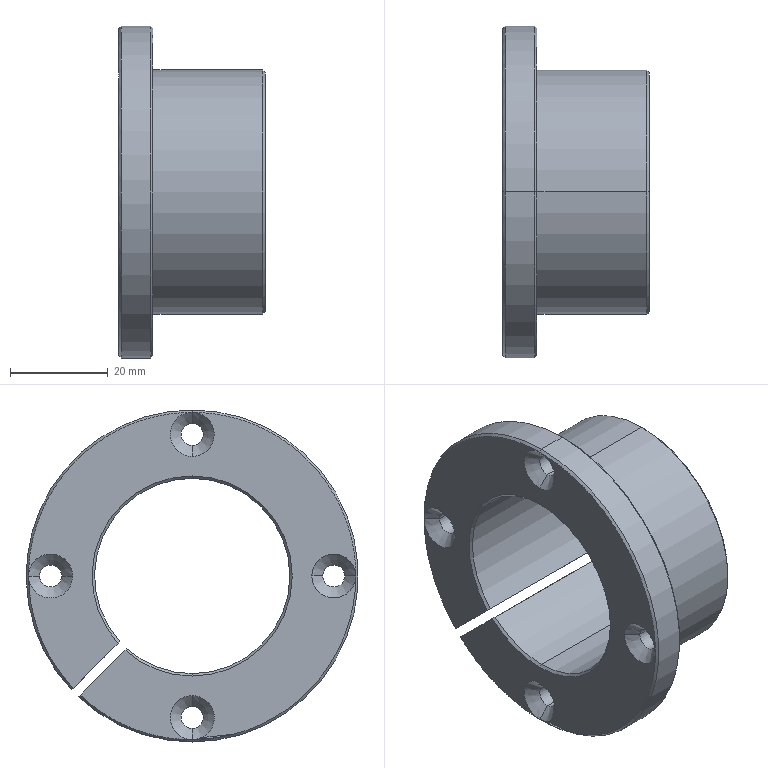Part | SolidWorks | features ICE 2, MoveFace 2, Chamfer 1, CirPattern 1, DelFace 1, RevCut 1, Revolution 1 | 1 solid | 45 faces | box 30 x 68 x 68 mm | volume 31718 mm3 | cone 23 | cylinder 17 | plane 5 | commonest cylinder face diameters 4.5 x8 40 x3 50 x3 68 x3
STEP:
#1=CARTESIAN_POINT('',(25.,0.,-24.5));
#2=VERTEX_POINT('',#1);
#3=CARTESIAN_POINT('',(25.,16.603,-18.017));
#4=VERTEX_POINT('',#3);
#5=CARTESIAN_POINT('',(25.,0.,0.));
#6=DIRECTION('',(1.,0.,0.));
#7=DIRECTION('',(0.,0.,-1.));
#8=AXIS2_PLACEMENT_3D('',#5,#6,#7);
#9=CIRCLE('',#8,24.5);
#10=EDGE_CURVE('',#2,#4,#9,.T.);
#11=ORIENTED_EDGE('',*,*,#10,.F.);
#12=CARTESIAN_POINT('',(24.5,0.,-25.));
#13=VERTEX_POINT('',#12);
#14=CARTESIAN_POINT('',(24.5,0.,-25.));
#15=DIRECTION('',(-0.7071,0.,-0.7071));
#16=VECTOR('',#15,1000.);
#17=LINE('',#14,#16);
#18=EDGE_CURVE('',#2,#13,#17,.T.);
#19=ORIENTED_EDGE('',*,*,#18,.T.);
#20=CARTESIAN_POINT('',(24.5,16.956,-18.371));
#21=VERTEX_POINT('',#20);
#22=CARTESIAN_POINT('',(24.5,0.,0.));
#23=DIRECTION('',(-1.,0.,0.));
#24=DIRECTION('',(0.,0.,-1.));
#25=AXIS2_PLACEMENT_3D('',#22,#23,#24);
#26=CIRCLE('',#25,25.);
#27=EDGE_CURVE('',#21,#13,#26,.T.);
#28=ORIENTED_EDGE('',*,*,#27,.F.);
#29=CARTESIAN_POINT('',(25.,16.603,-18.017));
#30=CARTESIAN_POINT('',(24.833,16.721,-18.135));
#31=CARTESIAN_POINT('',(24.667,16.838,-18.253));
#32=CARTESIAN_POINT('',(24.5,16.956,-18.371));
#33=B_SPLINE_CURVE_WITH_KNOTS('',3,(#29,#30,#31,#32),.UNSPECIFIED.,.F.,.F.,(4,4),(0.,0.0007074),.UNSPECIFIED.);
#34=EDGE_CURVE('',#4,#21,#33,.T.);
#35=ORIENTED_EDGE('',*,*,#34,.F.);
#36=EDGE_LOOP('',(#11,#19,#28,#35));
#37=FACE_OUTER_BOUND('',#36,.T.);
#38=CARTESIAN_POINT('',(24.5,0.,0.));
#39=DIRECTION('',(-1.,0.,0.));
#40=DIRECTION('',(0.,0.,1.));
#41=AXIS2_PLACEMENT_3D('',#38,#39,#40);
#42=CONICAL_SURFACE('',#41,25.,0.7854);
#43=ADVANCED_FACE('',(#37),#42,.T.);
#44=ORIENTED_EDGE('',*,*,#18,.F.);
#45=CARTESIAN_POINT('',(25.,0.,24.5));
#46=VERTEX_POINT('',#45);
#47=CARTESIAN_POINT('',(25.,0.,0.));
#48=DIRECTION('',(1.,0.,0.));
#49=DIRECTION('',(0.,0.,-1.));
#50=AXIS2_PLACEMENT_3D('',#47,#48,#49);
#51=CIRCLE('',#50,24.5);
#52=EDGE_CURVE('',#46,#2,#51,.T.);
#53=ORIENTED_EDGE('',*,*,#52,.F.);
#54=CARTESIAN_POINT('',(24.5,0.,25.));
#55=VERTEX_POINT('',#54);
#56=CARTESIAN_POINT('',(24.5,0.,25.));
#57=DIRECTION('',(-0.7071,0.,0.7071));
#58=VECTOR('',#57,1000.);
#59=LINE('',#56,#58);
#60=EDGE_CURVE('',#46,#55,#59,.T.);
#61=ORIENTED_EDGE('',*,*,#60,.T.);
#62=CARTESIAN_POINT('',(24.5,0.,0.));
#63=DIRECTION('',(-1.,0.,0.));
#64=DIRECTION('',(0.,0.,-1.));
#65=AXIS2_PLACEMENT_3D('',#62,#63,#64);
#66=CIRCLE('',#65,25.);
#67=EDGE_CURVE('',#13,#55,#66,.T.);
#68=ORIENTED_EDGE('',*,*,#67,.F.);
#69=EDGE_LOOP('',(#44,#53,#61,#68));
#70=FACE_OUTER_BOUND('',#69,.T.);
#71=CARTESIAN_POINT('',(24.5,0.,0.));
#72=DIRECTION('',(-1.,0.,0.));
#73=DIRECTION('',(0.,0.,1.));
#74=AXIS2_PLACEMENT_3D('',#71,#72,#73);
#75=CONICAL_SURFACE('',#74,25.,0.7854);
#76=ADVANCED_FACE('',(#70),#75,.T.);
#77=CARTESIAN_POINT('',(24.5,0.,20.));
#78=VERTEX_POINT('',#77);
#79=CARTESIAN_POINT('',(24.5,0.,-20.));
#80=VERTEX_POINT('',#79);
#81=CARTESIAN_POINT('',(24.5,0.,0.));
#82=DIRECTION('',(1.,0.,0.));
#83=DIRECTION('',(0.,0.,-1.));
#84=AXIS2_PLACEMENT_3D('',#81,#82,#83);
#85=CIRCLE('',#84,20.);
#86=EDGE_CURVE('',#78,#80,#85,.T.);
#87=ORIENTED_EDGE('',*,*,#86,.F.);
#88=CARTESIAN_POINT('',(25.,0.,20.5));
#89=VERTEX_POINT('',#88);
#90=CARTESIAN_POINT('',(24.5,0.,20.));
#91=DIRECTION('',(0.7071,0.,0.7071));
#92=VECTOR('',#91,1000.);
#93=LINE('',#90,#92);
#94=EDGE_CURVE('',#78,#89,#93,.T.);
#95=ORIENTED_EDGE('',*,*,#94,.T.);
#96=CARTESIAN_POINT('',(25.,0.,-20.5));
#97=VERTEX_POINT('',#96);
#98=CARTESIAN_POINT('',(25.,0.,0.));
#99=DIRECTION('',(-1.,0.,0.));
#100=DIRECTION('',(0.,0.,-1.));
#101=AXIS2_PLACEMENT_3D('',#98,#99,#100);
#102=CIRCLE('',#101,20.5);
#103=EDGE_CURVE('',#97,#89,#102,.T.);
#104=ORIENTED_EDGE('',*,*,#103,.F.);
#105=CARTESIAN_POINT('',(24.5,0.,-20.));
#106=DIRECTION('',(0.7071,0.,-0.7071));
#107=VECTOR('',#106,1000.);
#108=LINE('',#105,#107);
#109=EDGE_CURVE('',#80,#97,#108,.T.);
#110=ORIENTED_EDGE('',*,*,#109,.F.);
#111=EDGE_LOOP('',(#87,#95,#104,#110));
#112=FACE_OUTER_BOUND('',#111,.T.);
#113=CARTESIAN_POINT('',(24.5,0.,0.));
#114=DIRECTION('',(1.,0.,0.));
#115=DIRECTION('',(0.,0.,-1.));
#116=AXIS2_PLACEMENT_3D('',#113,#114,#115);
#117=CONICAL_SURFACE('',#116,20.,0.7854);
#118=ADVANCED_FACE('',(#112),#117,.F.);
#119=CARTESIAN_POINT('',(24.5,13.417,-14.832));
#120=VERTEX_POINT('',#119);
#121=CARTESIAN_POINT('',(24.5,0.,0.));
#122=DIRECTION('',(1.,0.,0.));
#123=DIRECTION('',(0.,0.,-1.));
#124=AXIS2_PLACEMENT_3D('',#121,#122,#123);
#125=CIRCLE('',#124,20.);
#126=EDGE_CURVE('',#80,#120,#125,.T.);
#127=ORIENTED_EDGE('',*,*,#126,.F.);
#128=ORIENTED_EDGE('',*,*,#109,.T.);
#129=CARTESIAN_POINT('',(25.,13.771,-15.186));
#130=VERTEX_POINT('',#129);
#131=CARTESIAN_POINT('',(25.,0.,0.));
#132=DIRECTION('',(-1.,0.,0.));
#133=DIRECTION('',(0.,0.,-1.));
#134=AXIS2_PLACEMENT_3D('',#131,#132,#133);
#135=CIRCLE('',#134,20.5);
#136=EDGE_CURVE('',#130,#97,#135,.T.);
#137=ORIENTED_EDGE('',*,*,#136,.F.);
#138=CARTESIAN_POINT('',(24.5,13.417,-14.832));
#139=CARTESIAN_POINT('',(24.667,13.535,-14.95));
#140=CARTESIAN_POINT('',(24.833,13.653,-15.068));
#141=CARTESIAN_POINT('',(25.,13.771,-15.186));
#142=B_SPLINE_CURVE_WITH_KNOTS('',3,(#138,#139,#140,#141),.UNSPECIFIED.,.F.,.F.,(4,4),(0.,0.0007075),.UNSPECIFIED.);
#143=EDGE_CURVE('',#120,#130,#142,.T.);
#144=ORIENTED_EDGE('',*,*,#143,.F.);
#145=EDGE_LOOP('',(#127,#128,#137,#144));
#146=FACE_OUTER_BOUND('',#145,.T.);
#147=CARTESIAN_POINT('',(24.5,0.,0.));
#148=DIRECTION('',(1.,0.,0.));
#149=DIRECTION('',(0.,0.,-1.));
#150=AXIS2_PLACEMENT_3D('',#147,#148,#149);
#151=CONICAL_SURFACE('',#150,20.,0.7854);
#152=ADVANCED_FACE('',(#146),#151,.F.);
#153=CARTESIAN_POINT('',(2.,0.,-33.5));
#154=VERTEX_POINT('',#153);
#155=CARTESIAN_POINT('',(2.,22.97,-24.385));
#156=VERTEX_POINT('',#155);
#157=CARTESIAN_POINT('',(2.,0.,0.));
#158=DIRECTION('',(1.,0.,0.));
#159=DIRECTION('',(0.,0.,-1.));
#160=AXIS2_PLACEMENT_3D('',#157,#158,#159);
#161=CIRCLE('',#160,33.5);
#162=EDGE_CURVE('',#154,#156,#161,.T.);
#163=ORIENTED_EDGE('',*,*,#162,.F.);
#164=CARTESIAN_POINT('',(1.5,0.,-34.));
#165=VERTEX_POINT('',#164);
#166=CARTESIAN_POINT('',(2.,0.,-33.5));
#167=DIRECTION('',(-0.7071,0.,-0.7071));
#168=VECTOR('',#167,1000.);
#169=LINE('',#166,#168);
#170=EDGE_CURVE('',#154,#165,#169,.T.);
#171=ORIENTED_EDGE('',*,*,#170,.T.);
#172=CARTESIAN_POINT('',(1.5,23.324,-24.738));
#173=VERTEX_POINT('',#172);
#174=CARTESIAN_POINT('',(1.5,0.,0.));
#175=DIRECTION('',(-1.,0.,0.));
#176=DIRECTION('',(0.,0.,-1.));
#177=AXIS2_PLACEMENT_3D('',#174,#175,#176);
#178=CIRCLE('',#177,34.);
#179=EDGE_CURVE('',#173,#165,#178,.T.);
#180=ORIENTED_EDGE('',*,*,#179,.F.);
#181=CARTESIAN_POINT('',(2.,22.97,-24.385));
#182=CARTESIAN_POINT('',(1.833,23.088,-24.503));
#183=CARTESIAN_POINT('',(1.667,23.206,-24.62));
#184=CARTESIAN_POINT('',(1.5,23.324,-24.738));
#185=B_SPLINE_CURVE_WITH_KNOTS('',3,(#181,#182,#183,#184),.UNSPECIFIED.,.F.,.F.,(4,4),(0.,0.0007073),.UNSPECIFIED.);
#186=EDGE_CURVE('',#156,#173,#185,.T.);
#187=ORIENTED_EDGE('',*,*,#186,.F.);
#188=EDGE_LOOP('',(#163,#171,#180,#187));
#189=FACE_OUTER_BOUND('',#188,.T.);
#190=CARTESIAN_POINT('',(2.,0.,0.));
#191=DIRECTION('',(-1.,0.,0.));
#192=DIRECTION('',(0.,0.,1.));
#193=AXIS2_PLACEMENT_3D('',#190,#191,#192);
#194=CONICAL_SURFACE('',#193,33.5,0.7854);
#195=ADVANCED_FACE('',(#189),#194,.T.);
#196=ORIENTED_EDGE('',*,*,#170,.F.);
#197=CARTESIAN_POINT('',(2.,0.,33.5));
#198=VERTEX_POINT('',#197);
#199=CARTESIAN_POINT('',(2.,0.,0.));
#200=DIRECTION('',(1.,0.,0.));
#201=DIRECTION('',(0.,0.,-1.));
#202=AXIS2_PLACEMENT_3D('',#199,#200,#201);
#203=CIRCLE('',#202,33.5);
#204=EDGE_CURVE('',#198,#154,#203,.T.);
#205=ORIENTED_EDGE('',*,*,#204,.F.);
#206=CARTESIAN_POINT('',(1.5,0.,34.));
#207=VERTEX_POINT('',#206);
#208=CARTESIAN_POINT('',(2.,0.,33.5));
#209=DIRECTION('',(-0.7071,0.,0.7071));
#210=VECTOR('',#209,1000.);
#211=LINE('',#208,#210);
#212=EDGE_CURVE('',#198,#207,#211,.T.);
#213=ORIENTED_EDGE('',*,*,#212,.T.);
#214=CARTESIAN_POINT('',(1.5,0.,0.));
#215=DIRECTION('',(-1.,0.,0.));
#216=DIRECTION('',(0.,0.,-1.));
#217=AXIS2_PLACEMENT_3D('',#214,#215,#216);
#218=CIRCLE('',#217,34.);
#219=EDGE_CURVE('',#165,#207,#218,.T.);
#220=ORIENTED_EDGE('',*,*,#219,.F.);
#221=EDGE_LOOP('',(#196,#205,#213,#220));
#222=FACE_OUTER_BOUND('',#221,.T.);
#223=CARTESIAN_POINT('',(2.,0.,0.));
#224=DIRECTION('',(-1.,0.,0.));
#225=DIRECTION('',(0.,0.,1.));
#226=AXIS2_PLACEMENT_3D('',#223,#224,#225);
#227=CONICAL_SURFACE('',#226,33.5,0.7854);
#228=ADVANCED_FACE('',(#222),#227,.T.);
#229=CARTESIAN_POINT('',(-5.,0.,33.5));
#230=VERTEX_POINT('',#229);
#231=CARTESIAN_POINT('',(-5.,33.5,0.));
#232=VERTEX_POINT('',#231);
#233=CARTESIAN_POINT('',(-5.,0.,0.));
#234=DIRECTION('',(-1.,0.,0.));
#235=DIRECTION('',(0.,0.,1.));
#236=AXIS2_PLACEMENT_3D('',#233,#234,#235);
#237=CIRCLE('',#236,33.5);
#238=EDGE_CURVE('',#230,#232,#237,.T.);
#239=ORIENTED_EDGE('',*,*,#238,.F.);
#240=CARTESIAN_POINT('',(-4.5,0.,34.));
#241=VERTEX_POINT('',#240);
#242=CARTESIAN_POINT('',(-5.,0.,33.5));
#243=DIRECTION('',(0.7071,0.,0.7071));
#244=VECTOR('',#243,1000.);
#245=LINE('',#242,#244);
#246=EDGE_CURVE('',#230,#241,#245,.T.);
#247=ORIENTED_EDGE('',*,*,#246,.T.);
#248=CARTESIAN_POINT('',(-4.5,24.738,-23.324));
#249=VERTEX_POINT('',#248);
#250=CARTESIAN_POINT('',(-4.5,0.,0.));
#251=DIRECTION('',(1.,0.,0.));
#252=DIRECTION('',(0.,0.,1.));
#253=AXIS2_PLACEMENT_3D('',#250,#251,#252);
#254=CIRCLE('',#253,34.);
#255=EDGE_CURVE('',#249,#241,#254,.T.);
#256=ORIENTED_EDGE('',*,*,#255,.F.);
#257=CARTESIAN_POINT('',(-5.,24.385,-22.97));
#258=VERTEX_POINT('',#257);
#259=CARTESIAN_POINT('',(-5.,24.385,-22.97));
#260=CARTESIAN_POINT('',(-4.833,24.503,-23.088));
#261=CARTESIAN_POINT('',(-4.667,24.62,-23.206));
#262=CARTESIAN_POINT('',(-4.5,24.738,-23.324));
#263=B_SPLINE_CURVE_WITH_KNOTS('',3,(#259,#260,#261,#262),.UNSPECIFIED.,.F.,.F.,(4,4),(0.,0.0007073),.UNSPECIFIED.);
#264=EDGE_CURVE('',#258,#249,#263,.T.);
#265=ORIENTED_EDGE('',*,*,#264,.F.);
#266=CARTESIAN_POINT('',(-5.,0.,0.));
#267=DIRECTION('',(-1.,0.,0.));
#268=DIRECTION('',(0.,0.,1.));
#269=AXIS2_PLACEMENT_3D('',#266,#267,#268);
#270=CIRCLE('',#269,33.5);
#271=EDGE_CURVE('',#232,#258,#270,.T.);
#272=ORIENTED_EDGE('',*,*,#271,.F.);
#273=EDGE_LOOP('',(#239,#247,#256,#265,#272));
#274=FACE_OUTER_BOUND('',#273,.T.);
#275=CARTESIAN_POINT('',(-5.,0.,0.));
#276=DIRECTION('',(1.,0.,0.));
#277=DIRECTION('',(0.,0.,-1.));
#278=AXIS2_PLACEMENT_3D('',#275,#276,#277);
#279=CONICAL_SURFACE('',#278,33.5,0.7854);
#280=ADVANCED_FACE('',(#274),#279,.T.);
#281=ORIENTED_EDGE('',*,*,#246,.F.);
#282=CARTESIAN_POINT('',(-5.,-33.5,0.));
#283=VERTEX_POINT('',#282);
#284=CARTESIAN_POINT('',(-5.,0.,0.));
#285=DIRECTION('',(-1.,0.,0.));
#286=DIRECTION('',(0.,0.,1.));
#287=AXIS2_PLACEMENT_3D('',#284,#285,#286);
#288=CIRCLE('',#287,33.5);
#289=EDGE_CURVE('',#283,#230,#288,.T.);
#290=ORIENTED_EDGE('',*,*,#289,.F.);
#291=CARTESIAN_POINT('',(-5.,0.,-33.5));
#292=VERTEX_POINT('',#291);
#293=CARTESIAN_POINT('',(-5.,0.,0.));
#294=DIRECTION('',(-1.,0.,0.));
#295=DIRECTION('',(0.,0.,1.));
#296=AXIS2_PLACEMENT_3D('',#293,#294,#295);
#297=CIRCLE('',#296,33.5);
#298=EDGE_CURVE('',#292,#283,#297,.T.);
#299=ORIENTED_EDGE('',*,*,#298,.F.);
#300=CARTESIAN_POINT('',(-4.5,0.,-34.));
#301=VERTEX_POINT('',#300);
#302=CARTESIAN_POINT('',(-5.,0.,-33.5));
#303=DIRECTION('',(0.7071,0.,-0.7071));
#304=VECTOR('',#303,1000.);
#305=LINE('',#302,#304);
#306=EDGE_CURVE('',#292,#301,#305,.T.);
#307=ORIENTED_EDGE('',*,*,#306,.T.);
#308=CARTESIAN_POINT('',(-4.5,0.,0.));
#309=DIRECTION('',(1.,0.,0.));
#310=DIRECTION('',(0.,0.,1.));
#311=AXIS2_PLACEMENT_3D('',#308,#309,#310);
#312=CIRCLE('',#311,34.);
#313=EDGE_CURVE('',#241,#301,#312,.T.);
#314=ORIENTED_EDGE('',*,*,#313,.F.);
#315=EDGE_LOOP('',(#281,#290,#299,#307,#314));
#316=FACE_OUTER_BOUND('',#315,.T.);
#317=CARTESIAN_POINT('',(-5.,0.,0.));
#318=DIRECTION('',(1.,0.,0.));
#319=DIRECTION('',(0.,0.,-1.));
#320=AXIS2_PLACEMENT_3D('',#317,#318,#319);
#321=CONICAL_SURFACE('',#320,33.5,0.7854);
#322=ADVANCED_FACE('',(#316),#321,.T.);
#323=CARTESIAN_POINT('',(-4.5,0.,-20.));
#324=VERTEX_POINT('',#323);
#325=CARTESIAN_POINT('',(-4.5,0.,20.));
#326=VERTEX_POINT('',#325);
#327=CARTESIAN_POINT('',(-4.5,0.,0.));
#328=DIRECTION('',(-1.,0.,0.));
#329=DIRECTION('',(0.,0.,1.));
#330=AXIS2_PLACEMENT_3D('',#327,#328,#329);
#331=CIRCLE('',#330,20.);
#332=EDGE_CURVE('',#324,#326,#331,.T.);
#333=ORIENTED_EDGE('',*,*,#332,.F.);
#334=CARTESIAN_POINT('',(-5.,0.,-20.5));
#335=VERTEX_POINT('',#334);
#336=CARTESIAN_POINT('',(-4.5,0.,-20.));
#337=DIRECTION('',(-0.7071,0.,-0.7071));
#338=VECTOR('',#337,1000.);
#339=LINE('',#336,#338);
#340=EDGE_CURVE('',#324,#335,#339,.T.);
#341=ORIENTED_EDGE('',*,*,#340,.T.);
#342=CARTESIAN_POINT('',(-5.,0.,20.5));
#343=VERTEX_POINT('',#342);
#344=CARTESIAN_POINT('',(-5.,0.,0.));
#345=DIRECTION('',(1.,0.,0.));
#346=DIRECTION('',(0.,0.,1.));
#347=AXIS2_PLACEMENT_3D('',#344,#345,#346);
#348=CIRCLE('',#347,20.5);
#349=EDGE_CURVE('',#343,#335,#348,.T.);
#350=ORIENTED_EDGE('',*,*,#349,.F.);
#351=CARTESIAN_POINT('',(-4.5,0.,20.));
#352=DIRECTION('',(-0.7071,0.,0.7071));
#353=VECTOR('',#352,1000.);
#354=LINE('',#351,#353);
#355=EDGE_CURVE('',#326,#343,#354,.T.);
#356=ORIENTED_EDGE('',*,*,#355,.F.);
#357=EDGE_LOOP('',(#333,#341,#350,#356));
#358=FACE_OUTER_BOUND('',#357,.T.);
#359=CARTESIAN_POINT('',(-4.5,0.,0.));
#360=DIRECTION('',(-1.,0.,0.));
#361=DIRECTION('',(0.,0.,1.));
#362=AXIS2_PLACEMENT_3D('',#359,#360,#361);
#363=CONICAL_SURFACE('',#362,20.,0.7854);
#364=ADVANCED_FACE('',(#358),#363,.F.);
#365=CARTESIAN_POINT('',(-4.5,14.832,-13.417));
#366=VERTEX_POINT('',#365);
#367=CARTESIAN_POINT('',(-4.5,0.,0.));
#368=DIRECTION('',(-1.,0.,0.));
#369=DIRECTION('',(0.,0.,1.));
#370=AXIS2_PLACEMENT_3D('',#367,#368,#369);
#371=CIRCLE('',#370,20.);
#372=EDGE_CURVE('',#326,#366,#371,.T.);
#373=ORIENTED_EDGE('',*,*,#372,.F.);
#374=ORIENTED_EDGE('',*,*,#355,.T.);
#375=CARTESIAN_POINT('',(-5.,15.186,-13.771));
#376=VERTEX_POINT('',#375);
#377=CARTESIAN_POINT('',(-5.,0.,0.));
#378=DIRECTION('',(1.,0.,0.));
#379=DIRECTION('',(0.,0.,1.));
#380=AXIS2_PLACEMENT_3D('',#377,#378,#379);
#381=CIRCLE('',#380,20.5);
#382=EDGE_CURVE('',#376,#343,#381,.T.);
#383=ORIENTED_EDGE('',*,*,#382,.F.);
#384=CARTESIAN_POINT('',(-4.5,14.832,-13.417));
#385=CARTESIAN_POINT('',(-4.667,14.95,-13.535));
#386=CARTESIAN_POINT('',(-4.833,15.068,-13.653));
#387=CARTESIAN_POINT('',(-5.,15.186,-13.771));
#388=B_SPLINE_CURVE_WITH_KNOTS('',3,(#384,#385,#386,#387),.UNSPECIFIED.,.F.,.F.,(4,4),(0.,0.0007075),.UNSPECIFIED.);
#389=EDGE_CURVE('',#366,#376,#388,.T.);
#390=ORIENTED_EDGE('',*,*,#389,.F.);
#391=EDGE_LOOP('',(#373,#374,#383,#390));
#392=FACE_OUTER_BOUND('',#391,.T.);
#393=CARTESIAN_POINT('',(-4.5,0.,0.));
#394=DIRECTION('',(-1.,0.,0.));
#395=DIRECTION('',(0.,0.,1.));
#396=AXIS2_PLACEMENT_3D('',#393,#394,#395);
#397=CONICAL_SURFACE('',#396,20.,0.7854);
#398=ADVANCED_FACE('',(#392),#397,.F.);
#399=ORIENTED_EDGE('',*,*,#179,.T.);
#400=CARTESIAN_POINT('',(5.,0.,-34.));
#401=DIRECTION('',(-1.,0.,0.));
#402=VECTOR('',#401,1000.);
#403=LINE('',#400,#402);
#404=EDGE_CURVE('',#165,#301,#403,.T.);
#405=ORIENTED_EDGE('',*,*,#404,.T.);
#406=CARTESIAN_POINT('',(-4.5,23.324,-24.738));
#407=VERTEX_POINT('',#406);
#408=CARTESIAN_POINT('',(-4.5,0.,0.));
#409=DIRECTION('',(1.,0.,0.));
#410=DIRECTION('',(0.,0.,1.));
#411=AXIS2_PLACEMENT_3D('',#408,#409,#410);
#412=CIRCLE('',#411,34.);
#413=EDGE_CURVE('',#301,#407,#412,.T.);
#414=ORIENTED_EDGE('',*,*,#413,.T.);
#415=CARTESIAN_POINT('',(5.,23.324,-24.738));
#416=DIRECTION('',(1.,0.,0.));
#417=VECTOR('',#416,1000.);
#418=LINE('',#415,#417);
#419=EDGE_CURVE('',#407,#173,#418,.T.);
#420=ORIENTED_EDGE('',*,*,#419,.T.);
#421=EDGE_LOOP('',(#399,#405,#414,#420));
#422=FACE_OUTER_BOUND('',#421,.T.);
#423=CARTESIAN_POINT('',(5.,0.,0.));
#424=DIRECTION('',(-1.,0.,0.));
#425=DIRECTION('',(0.,0.,1.));
#426=AXIS2_PLACEMENT_3D('',#423,#424,#425);
#427=CYLINDRICAL_SURFACE('',#426,34.);
#428=ADVANCED_FACE('',(#422),#427,.T.);
#429=ORIENTED_EDGE('',*,*,#404,.F.);
#430=ORIENTED_EDGE('',*,*,#219,.T.);
#431=CARTESIAN_POINT('',(5.,0.,34.));
#432=DIRECTION('',(-1.,0.,0.));
#433=VECTOR('',#432,1000.);
#434=LINE('',#431,#433);
#435=EDGE_CURVE('',#207,#241,#434,.T.);
#436=ORIENTED_EDGE('',*,*,#435,.T.);
#437=ORIENTED_EDGE('',*,*,#313,.T.);
#438=EDGE_LOOP('',(#429,#430,#436,#437));
#439=FACE_OUTER_BOUND('',#438,.T.);
#440=CARTESIAN_POINT('',(5.,0.,0.));
#441=DIRECTION('',(-1.,0.,0.));
#442=DIRECTION('',(0.,0.,1.));
#443=AXIS2_PLACEMENT_3D('',#440,#441,#442);
#444=CYLINDRICAL_SURFACE('',#443,34.);
#445=ADVANCED_FACE('',(#439),#444,.T.);
#446=CARTESIAN_POINT('',(-2.75,31.25,0.));
#447=VERTEX_POINT('',#446);
#448=CARTESIAN_POINT('',(-2.75,26.75,0.));
#449=VERTEX_POINT('',#448);
#450=CARTESIAN_POINT('',(-2.75,29.,0.));
#451=DIRECTION('',(-1.,0.,0.));
#452=DIRECTION('',(0.,-1.,0.));
#453=AXIS2_PLACEMENT_3D('',#450,#451,#452);
#454=CIRCLE('',#453,2.25);
#455=EDGE_CURVE('',#447,#449,#454,.T.);
#456=ORIENTED_EDGE('',*,*,#455,.F.);
#457=CARTESIAN_POINT('',(-2.75,31.25,0.));
#458=DIRECTION('',(-0.7071,0.7071,0.));
#459=VECTOR('',#458,1000.);
#460=LINE('',#457,#459);
#461=EDGE_CURVE('',#447,#232,#460,.T.);
#462=ORIENTED_EDGE('',*,*,#461,.T.);
#463=CARTESIAN_POINT('',(-5.,24.5,0.));
#464=VERTEX_POINT('',#463);
#465=CARTESIAN_POINT('',(-5.,29.,0.));
#466=DIRECTION('',(-1.,0.,0.));
#467=DIRECTION('',(0.,-1.,0.));
#468=AXIS2_PLACEMENT_3D('',#465,#466,#467);
#469=CIRCLE('',#468,4.5);
#470=EDGE_CURVE('',#232,#464,#469,.T.);
#471=ORIENTED_EDGE('',*,*,#470,.T.);
#472=CARTESIAN_POINT('',(-2.75,26.75,0.));
#473=DIRECTION('',(-0.7071,-0.7071,0.));
#474=VECTOR('',#473,1000.);
#475=LINE('',#472,#474);
#476=EDGE_CURVE('',#449,#464,#475,.T.);
#477=ORIENTED_EDGE('',*,*,#476,.F.);
#478=EDGE_LOOP('',(#456,#462,#471,#477));
#479=FACE_OUTER_BOUND('',#478,.T.);
#480=CARTESIAN_POINT('',(-2.75,29.,0.));
#481=DIRECTION('',(-1.,0.,0.));
#482=DIRECTION('',(0.,-1.,0.));
#483=AXIS2_PLACEMENT_3D('',#480,#481,#482);
#484=CONICAL_SURFACE('',#483,2.25,0.7854);
#485=ADVANCED_FACE('',(#479),#484,.F.);
#486=CARTESIAN_POINT('',(2.,31.25,0.));
#487=VERTEX_POINT('',#486);
#488=CARTESIAN_POINT('',(2.,26.75,0.));
#489=VERTEX_POINT('',#488);
#490=CARTESIAN_POINT('',(2.,29.,0.));
#491=DIRECTION('',(-1.,0.,0.));
#492=DIRECTION('',(0.,-1.,0.));
#493=AXIS2_PLACEMENT_3D('',#490,#491,#492);
#494=CIRCLE('',#493,2.25);
#495=EDGE_CURVE('',#487,#489,#494,.T.);
#496=ORIENTED_EDGE('',*,*,#495,.F.);
#497=CARTESIAN_POINT('',(-5.,31.25,0.));
#498=DIRECTION('',(-1.,0.,0.));
#499=VECTOR('',#498,1000.);
#500=LINE('',#497,#499);
#501=EDGE_CURVE('',#487,#447,#500,.T.);
#502=ORIENTED_EDGE('',*,*,#501,.T.);
#503=ORIENTED_EDGE('',*,*,#455,.T.);
#504=CARTESIAN_POINT('',(-5.,26.75,0.));
#505=DIRECTION('',(-1.,0.,0.));
#506=VECTOR('',#505,1000.);
#507=LINE('',#504,#506);
#508=EDGE_CURVE('',#489,#449,#507,.T.);
#509=ORIENTED_EDGE('',*,*,#508,.F.);
#510=EDGE_LOOP('',(#496,#502,#503,#509));
#511=FACE_OUTER_BOUND('',#510,.T.);
#512=CARTESIAN_POINT('',(-5.,29.,0.));
#513=DIRECTION('',(-1.,0.,0.));
#514=DIRECTION('',(0.,-1.,0.));
#515=AXIS2_PLACEMENT_3D('',#512,#513,#514);
#516=CYLINDRICAL_SURFACE('',#515,2.25);
#517=ADVANCED_FACE('',(#511),#516,.F.);
#518=CARTESIAN_POINT('',(-2.75,0.,31.25));
#519=VERTEX_POINT('',#518);
#520=CARTESIAN_POINT('',(-2.75,0.,26.75));
#521=VERTEX_POINT('',#520);
#522=CARTESIAN_POINT('',(-2.75,0.,29.));
#523=DIRECTION('',(-1.,0.,0.));
#524=DIRECTION('',(0.,0.,-1.));
#525=AXIS2_PLACEMENT_3D('',#522,#523,#524);
#526=CIRCLE('',#525,2.25);
#527=EDGE_CURVE('',#519,#521,#526,.T.);
#528=ORIENTED_EDGE('',*,*,#527,.F.);
#529=CARTESIAN_POINT('',(-2.75,0.,31.25));
#530=DIRECTION('',(-0.7071,0.,0.7071));
#531=VECTOR('',#530,1000.);
#532=LINE('',#529,#531);
#533=EDGE_CURVE('',#519,#230,#532,.T.);
#534=ORIENTED_EDGE('',*,*,#533,.T.);
#535=CARTESIAN_POINT('',(-5.,0.,24.5));
#536=VERTEX_POINT('',#535);
#537=CARTESIAN_POINT('',(-5.,0.,29.));
#538=DIRECTION('',(-1.,0.,0.));
#539=DIRECTION('',(0.,0.,-1.));
#540=AXIS2_PLACEMENT_3D('',#537,#538,#539);
#541=CIRCLE('',#540,4.5);
#542=EDGE_CURVE('',#230,#536,#541,.T.);
#543=ORIENTED_EDGE('',*,*,#542,.T.);
#544=CARTESIAN_POINT('',(-2.75,0.,26.75));
#545=DIRECTION('',(-0.7071,0.,-0.7071));
#546=VECTOR('',#545,1000.);
#547=LINE('',#544,#546);
#548=EDGE_CURVE('',#521,#536,#547,.T.);
#549=ORIENTED_EDGE('',*,*,#548,.F.);
#550=EDGE_LOOP('',(#528,#534,#543,#549));
#551=FACE_OUTER_BOUND('',#550,.T.);
#552=CARTESIAN_POINT('',(-2.75,0.,29.));
#553=DIRECTION('',(-1.,0.,0.));
#554=DIRECTION('',(0.,0.,-1.));
#555=AXIS2_PLACEMENT_3D('',#552,#553,#554);
#556=CONICAL_SURFACE('',#555,2.25,0.7854);
#557=ADVANCED_FACE('',(#551),#556,.F.);
#558=CARTESIAN_POINT('',(2.,0.,31.25));
#559=VERTEX_POINT('',#558);
#560=CARTESIAN_POINT('',(2.,0.,26.75));
#561=VERTEX_POINT('',#560);
#562=CARTESIAN_POINT('',(2.,0.,29.));
#563=DIRECTION('',(-1.,0.,0.));
#564=DIRECTION('',(0.,0.,-1.));
#565=AXIS2_PLACEMENT_3D('',#562,#563,#564);
#566=CIRCLE('',#565,2.25);
#567=EDGE_CURVE('',#559,#561,#566,.T.);
#568=ORIENTED_EDGE('',*,*,#567,.F.);
#569=CARTESIAN_POINT('',(-5.,0.,31.25));
#570=DIRECTION('',(-1.,0.,0.));
#571=VECTOR('',#570,1000.);
#572=LINE('',#569,#571);
#573=EDGE_CURVE('',#559,#519,#572,.T.);
#574=ORIENTED_EDGE('',*,*,#573,.T.);
#575=ORIENTED_EDGE('',*,*,#527,.T.);
#576=CARTESIAN_POINT('',(-5.,0.,26.75));
#577=DIRECTION('',(-1.,0.,0.));
#578=VECTOR('',#577,1000.);
#579=LINE('',#576,#578);
#580=EDGE_CURVE('',#561,#521,#579,.T.);
#581=ORIENTED_EDGE('',*,*,#580,.F.);
#582=EDGE_LOOP('',(#568,#574,#575,#581));
#583=FACE_OUTER_BOUND('',#582,.T.);
#584=CARTESIAN_POINT('',(-5.,0.,29.));
#585=DIRECTION('',(-1.,0.,0.));
#586=DIRECTION('',(0.,0.,-1.));
#587=AXIS2_PLACEMENT_3D('',#584,#585,#586);
#588=CYLINDRICAL_SURFACE('',#587,2.25);
#589=ADVANCED_FACE('',(#583),#588,.F.);
#590=CARTESIAN_POINT('',(-2.75,-31.25,0.));
#591=VERTEX_POINT('',#590);
#592=CARTESIAN_POINT('',(-2.75,-26.75,0.));
#593=VERTEX_POINT('',#592);
#594=CARTESIAN_POINT('',(-2.75,-29.,0.));
#595=DIRECTION('',(-1.,0.,0.));
#596=DIRECTION('',(0.,1.,0.));
#597=AXIS2_PLACEMENT_3D('',#594,#595,#596);
#598=CIRCLE('',#597,2.25);
#599=EDGE_CURVE('',#591,#593,#598,.T.);
#600=ORIENTED_EDGE('',*,*,#599,.F.);
#601=CARTESIAN_POINT('',(-2.75,-31.25,0.));
#602=DIRECTION('',(-0.7071,-0.7071,0.));
#603=VECTOR('',#602,1000.);
#604=LINE('',#601,#603);
#605=EDGE_CURVE('',#591,#283,#604,.T.);
#606=ORIENTED_EDGE('',*,*,#605,.T.);
#607=CARTESIAN_POINT('',(-5.,-24.5,0.));
#608=VERTEX_POINT('',#607);
#609=CARTESIAN_POINT('',(-5.,-29.,0.));
#610=DIRECTION('',(-1.,0.,0.));
#611=DIRECTION('',(0.,1.,0.));
#612=AXIS2_PLACEMENT_3D('',#609,#610,#611);
#613=CIRCLE('',#612,4.5);
#614=EDGE_CURVE('',#283,#608,#613,.T.);
#615=ORIENTED_EDGE('',*,*,#614,.T.);
#616=CARTESIAN_POINT('',(-2.75,-26.75,0.));
#617=DIRECTION('',(-0.7071,0.7071,0.));
#618=VECTOR('',#617,1000.);
#619=LINE('',#616,#618);
#620=EDGE_CURVE('',#593,#608,#619,.T.);
#621=ORIENTED_EDGE('',*,*,#620,.F.);
#622=EDGE_LOOP('',(#600,#606,#615,#621));
#623=FACE_OUTER_BOUND('',#622,.T.);
#624=CARTESIAN_POINT('',(-2.75,-29.,0.));
#625=DIRECTION('',(-1.,0.,0.));
#626=DIRECTION('',(0.,1.,0.));
#627=AXIS2_PLACEMENT_3D('',#624,#625,#626);
#628=CONICAL_SURFACE('',#627,2.25,0.7854);
#629=ADVANCED_FACE('',(#623),#628,.F.);
#630=CARTESIAN_POINT('',(2.,-31.25,0.));
#631=VERTEX_POINT('',#630);
#632=CARTESIAN_POINT('',(2.,-26.75,0.));
#633=VERTEX_POINT('',#632);
#634=CARTESIAN_POINT('',(2.,-29.,0.));
#635=DIRECTION('',(-1.,0.,0.));
#636=DIRECTION('',(0.,1.,0.));
#637=AXIS2_PLACEMENT_3D('',#634,#635,#636);
#638=CIRCLE('',#637,2.25);
#639=EDGE_CURVE('',#631,#633,#638,.T.);
#640=ORIENTED_EDGE('',*,*,#639,.F.);
#641=CARTESIAN_POINT('',(-5.,-31.25,0.));
#642=DIRECTION('',(-1.,0.,0.));
#643=VECTOR('',#642,1000.);
#644=LINE('',#641,#643);
#645=EDGE_CURVE('',#631,#591,#644,.T.);
#646=ORIENTED_EDGE('',*,*,#645,.T.);
#647=ORIENTED_EDGE('',*,*,#599,.T.);
#648=CARTESIAN_POINT('',(-5.,-26.75,0.));
#649=DIRECTION('',(-1.,0.,0.));
#650=VECTOR('',#649,1000.);
#651=LINE('',#648,#650);
#652=EDGE_CURVE('',#633,#593,#651,.T.);
#653=ORIENTED_EDGE('',*,*,#652,.F.);
#654=EDGE_LOOP('',(#640,#646,#647,#653));
#655=FACE_OUTER_BOUND('',#654,.T.);
#656=CARTESIAN_POINT('',(-5.,-29.,0.));
#657=DIRECTION('',(-1.,0.,0.));
#658=DIRECTION('',(0.,1.,0.));
#659=AXIS2_PLACEMENT_3D('',#656,#657,#658);
#660=CYLINDRICAL_SURFACE('',#659,2.25);
#661=ADVANCED_FACE('',(#655),#660,.F.);
#662=CARTESIAN_POINT('',(-2.75,0.,-31.25));
#663=VERTEX_POINT('',#662);
#664=CARTESIAN_POINT('',(-2.75,0.,-26.75));
#665=VERTEX_POINT('',#664);
#666=CARTESIAN_POINT('',(-2.75,0.,-29.));
#667=DIRECTION('',(-1.,0.,0.));
#668=DIRECTION('',(0.,0.,1.));
#669=AXIS2_PLACEMENT_3D('',#666,#667,#668);
#670=CIRCLE('',#669,2.25);
#671=EDGE_CURVE('',#663,#665,#670,.T.);
#672=ORIENTED_EDGE('',*,*,#671,.F.);
#673=CARTESIAN_POINT('',(-2.75,0.,-31.25));
#674=DIRECTION('',(-0.7071,0.,-0.7071));
#675=VECTOR('',#674,1000.);
#676=LINE('',#673,#675);
#677=EDGE_CURVE('',#663,#292,#676,.T.);
#678=ORIENTED_EDGE('',*,*,#677,.T.);
#679=CARTESIAN_POINT('',(-5.,0.,-24.5));
#680=VERTEX_POINT('',#679);
#681=CARTESIAN_POINT('',(-5.,0.,-29.));
#682=DIRECTION('',(-1.,0.,0.));
#683=DIRECTION('',(0.,0.,1.));
#684=AXIS2_PLACEMENT_3D('',#681,#682,#683);
#685=CIRCLE('',#684,4.5);
#686=EDGE_CURVE('',#292,#680,#685,.T.);
#687=ORIENTED_EDGE('',*,*,#686,.T.);
#688=CARTESIAN_POINT('',(-2.75,0.,-26.75));
#689=DIRECTION('',(-0.7071,0.,0.7071));
#690=VECTOR('',#689,1000.);
#691=LINE('',#688,#690);
#692=EDGE_CURVE('',#665,#680,#691,.T.);
#693=ORIENTED_EDGE('',*,*,#692,.F.);
#694=EDGE_LOOP('',(#672,#678,#687,#693));
#695=FACE_OUTER_BOUND('',#694,.T.);
#696=CARTESIAN_POINT('',(-2.75,0.,-29.));
#697=DIRECTION('',(-1.,0.,0.));
#698=DIRECTION('',(0.,0.,1.));
#699=AXIS2_PLACEMENT_3D('',#696,#697,#698);
#700=CONICAL_SURFACE('',#699,2.25,0.7854);
#701=ADVANCED_FACE('',(#695),#700,.F.);
#702=CARTESIAN_POINT('',(2.,0.,-31.25));
#703=VERTEX_POINT('',#702);
#704=CARTESIAN_POINT('',(2.,0.,-26.75));
#705=VERTEX_POINT('',#704);
#706=CARTESIAN_POINT('',(2.,0.,-29.));
#707=DIRECTION('',(-1.,0.,0.));
#708=DIRECTION('',(0.,0.,1.));
#709=AXIS2_PLACEMENT_3D('',#706,#707,#708);
#710=CIRCLE('',#709,2.25);
#711=EDGE_CURVE('',#703,#705,#710,.T.);
#712=ORIENTED_EDGE('',*,*,#711,.F.);
#713=CARTESIAN_POINT('',(-5.,0.,-31.25));
#714=DIRECTION('',(-1.,0.,0.));
#715=VECTOR('',#714,1000.);
#716=LINE('',#713,#715);
#717=EDGE_CURVE('',#703,#663,#716,.T.);
#718=ORIENTED_EDGE('',*,*,#717,.T.);
#719=ORIENTED_EDGE('',*,*,#671,.T.);
#720=CARTESIAN_POINT('',(-5.,0.,-26.75));
#721=DIRECTION('',(-1.,0.,0.));
#722=VECTOR('',#721,1000.);
#723=LINE('',#720,#722);
#724=EDGE_CURVE('',#705,#665,#723,.T.);
#725=ORIENTED_EDGE('',*,*,#724,.F.);
#726=EDGE_LOOP('',(#712,#718,#719,#725));
#727=FACE_OUTER_BOUND('',#726,.T.);
#728=CARTESIAN_POINT('',(-5.,0.,-29.));
#729=DIRECTION('',(-1.,0.,0.));
#730=DIRECTION('',(0.,0.,1.));
#731=AXIS2_PLACEMENT_3D('',#728,#729,#730);
#732=CYLINDRICAL_SURFACE('',#731,2.25);
#733=ADVANCED_FACE('',(#727),#732,.F.);
#734=ORIENTED_EDGE('',*,*,#86,.T.);
#735=CARTESIAN_POINT('',(25.002,0.,-20.));
#736=DIRECTION('',(-1.,0.,0.));
#737=VECTOR('',#736,1000.);
#738=LINE('',#735,#737);
#739=EDGE_CURVE('',#80,#324,#738,.T.);
#740=ORIENTED_EDGE('',*,*,#739,.T.);
#741=ORIENTED_EDGE('',*,*,#332,.T.);
#742=CARTESIAN_POINT('',(25.002,0.,20.));
#743=DIRECTION('',(-1.,0.,0.));
#744=VECTOR('',#743,1000.);
#745=LINE('',#742,#744);
#746=EDGE_CURVE('',#78,#326,#745,.T.);
#747=ORIENTED_EDGE('',*,*,#746,.F.);
#748=EDGE_LOOP('',(#734,#740,#741,#747));
#749=FACE_OUTER_BOUND('',#748,.T.);
#750=CARTESIAN_POINT('',(25.002,0.,0.));
#751=DIRECTION('',(-1.,0.,0.));
#752=DIRECTION('',(0.,0.,1.));
#753=AXIS2_PLACEMENT_3D('',#750,#751,#752);
#754=CYLINDRICAL_SURFACE('',#753,20.);
#755=ADVANCED_FACE('',(#749),#754,.F.);
#756=CARTESIAN_POINT('',(24.5,14.832,-13.417));
#757=VERTEX_POINT('',#756);
#758=CARTESIAN_POINT('',(24.5,0.,0.));
#759=DIRECTION('',(1.,0.,0.));
#760=DIRECTION('',(0.,0.,-1.));
#761=AXIS2_PLACEMENT_3D('',#758,#759,#760);
#762=CIRCLE('',#761,20.);
#763=EDGE_CURVE('',#757,#78,#762,.T.);
#764=ORIENTED_EDGE('',*,*,#763,.T.);
#765=ORIENTED_EDGE('',*,*,#746,.T.);
#766=ORIENTED_EDGE('',*,*,#372,.T.);
#767=CARTESIAN_POINT('',(25.002,14.832,-13.417));
#768=DIRECTION('',(-1.,0.,0.));
#769=VECTOR('',#768,1000.);
#770=LINE('',#767,#769);
#771=EDGE_CURVE('',#757,#366,#770,.T.);
#772=ORIENTED_EDGE('',*,*,#771,.F.);
#773=EDGE_LOOP('',(#764,#765,#766,#772));
#774=FACE_OUTER_BOUND('',#773,.T.);
#775=CARTESIAN_POINT('',(25.002,0.,0.));
#776=DIRECTION('',(-1.,0.,0.));
#777=DIRECTION('',(0.,0.,1.));
#778=AXIS2_PLACEMENT_3D('',#775,#776,#777);
#779=CYLINDRICAL_SURFACE('',#778,20.);
#780=ADVANCED_FACE('',(#774),#779,.F.);
#781=ORIENTED_EDGE('',*,*,#27,.T.);
#782=CARTESIAN_POINT('',(2.,0.,-25.));
#783=VERTEX_POINT('',#782);
#784=CARTESIAN_POINT('',(25.002,0.,-25.));
#785=DIRECTION('',(-1.,0.,0.));
#786=VECTOR('',#785,1000.);
#787=LINE('',#784,#786);
#788=EDGE_CURVE('',#13,#783,#787,.T.);
#789=ORIENTED_EDGE('',*,*,#788,.T.);
#790=CARTESIAN_POINT('',(2.,16.956,-18.371));
#791=VERTEX_POINT('',#790);
#792=CARTESIAN_POINT('',(2.,0.,0.));
#793=DIRECTION('',(-1.,0.,0.));
#794=DIRECTION('',(0.,0.,1.));
#795=AXIS2_PLACEMENT_3D('',#792,#793,#794);
#796=CIRCLE('',#795,25.);
#797=EDGE_CURVE('',#791,#783,#796,.T.);
#798=ORIENTED_EDGE('',*,*,#797,.F.);
#799=CARTESIAN_POINT('',(25.002,16.956,-18.371));
#800=DIRECTION('',(-1.,0.,0.));
#801=VECTOR('',#800,1000.);
#802=LINE('',#799,#801);
#803=EDGE_CURVE('',#21,#791,#802,.T.);
#804=ORIENTED_EDGE('',*,*,#803,.F.);
#805=EDGE_LOOP('',(#781,#789,#798,#804));
#806=FACE_OUTER_BOUND('',#805,.T.);
#807=CARTESIAN_POINT('',(25.002,0.,0.));
#808=DIRECTION('',(-1.,0.,0.));
#809=DIRECTION('',(0.,0.,1.));
#810=AXIS2_PLACEMENT_3D('',#807,#808,#809);
#811=CYLINDRICAL_SURFACE('',#810,25.);
#812=ADVANCED_FACE('',(#806),#811,.T.);
#813=ORIENTED_EDGE('',*,*,#788,.F.);
#814=ORIENTED_EDGE('',*,*,#67,.T.);
#815=CARTESIAN_POINT('',(2.,0.,25.));
#816=VERTEX_POINT('',#815);
#817=CARTESIAN_POINT('',(25.002,0.,25.));
#818=DIRECTION('',(-1.,0.,0.));
#819=VECTOR('',#818,1000.);
#820=LINE('',#817,#819);
#821=EDGE_CURVE('',#55,#816,#820,.T.);
#822=ORIENTED_EDGE('',*,*,#821,.T.);
#823=CARTESIAN_POINT('',(2.,0.,0.));
#824=DIRECTION('',(-1.,0.,0.));
#825=DIRECTION('',(0.,0.,1.));
#826=AXIS2_PLACEMENT_3D('',#823,#824,#825);
#827=CIRCLE('',#826,25.);
#828=EDGE_CURVE('',#783,#816,#827,.T.);
#829=ORIENTED_EDGE('',*,*,#828,.F.);
#830=EDGE_LOOP('',(#813,#814,#822,#829));
#831=FACE_OUTER_BOUND('',#830,.T.);
#832=CARTESIAN_POINT('',(25.002,0.,0.));
#833=DIRECTION('',(-1.,0.,0.));
#834=DIRECTION('',(0.,0.,1.));
#835=AXIS2_PLACEMENT_3D('',#832,#833,#834);
#836=CYLINDRICAL_SURFACE('',#835,25.);
#837=ADVANCED_FACE('',(#831),#836,.T.);
#838=CARTESIAN_POINT('',(2.,29.,0.));
#839=DIRECTION('',(-1.,0.,0.));
#840=DIRECTION('',(0.,-1.,0.));
#841=AXIS2_PLACEMENT_3D('',#838,#839,#840);
#842=CIRCLE('',#841,2.25);
#843=EDGE_CURVE('',#489,#487,#842,.T.);
#844=ORIENTED_EDGE('',*,*,#843,.T.);
#845=ORIENTED_EDGE('',*,*,#495,.T.);
#846=EDGE_LOOP('',(#844,#845));
#847=FACE_BOUND('',#846,.T.);
#848=CARTESIAN_POINT('',(2.,0.,29.));
#849=DIRECTION('',(-1.,0.,0.));
#850=DIRECTION('',(0.,0.,-1.));
#851=AXIS2_PLACEMENT_3D('',#848,#849,#850);
#852=CIRCLE('',#851,2.25);
#853=EDGE_CURVE('',#561,#559,#852,.T.);
#854=ORIENTED_EDGE('',*,*,#853,.T.);
#855=ORIENTED_EDGE('',*,*,#567,.T.);
#856=EDGE_LOOP('',(#854,#855));
#857=FACE_BOUND('',#856,.T.);
#858=CARTESIAN_POINT('',(2.,-29.,0.));
#859=DIRECTION('',(-1.,0.,0.));
#860=DIRECTION('',(0.,1.,0.));
#861=AXIS2_PLACEMENT_3D('',#858,#859,#860);
#862=CIRCLE('',#861,2.25);
#863=EDGE_CURVE('',#633,#631,#862,.T.);
#864=ORIENTED_EDGE('',*,*,#863,.T.);
#865=ORIENTED_EDGE('',*,*,#639,.T.);
#866=EDGE_LOOP('',(#864,#865));
#867=FACE_BOUND('',#866,.T.);
#868=CARTESIAN_POINT('',(2.,0.,-29.));
#869=DIRECTION('',(-1.,0.,0.));
#870=DIRECTION('',(0.,0.,1.));
#871=AXIS2_PLACEMENT_3D('',#868,#869,#870);
#872=CIRCLE('',#871,2.25);
#873=EDGE_CURVE('',#705,#703,#872,.T.);
#874=ORIENTED_EDGE('',*,*,#873,.T.);
#875=ORIENTED_EDGE('',*,*,#711,.T.);
#876=EDGE_LOOP('',(#874,#875));
#877=FACE_BOUND('',#876,.T.);
#878=CARTESIAN_POINT('',(2.,24.385,-22.97));
#879=VERTEX_POINT('',#878);
#880=CARTESIAN_POINT('',(2.,18.371,-16.956));
#881=VERTEX_POINT('',#880);
#882=CARTESIAN_POINT('',(2.,18.207,-16.793));
#883=DIRECTION('',(0.,-0.7071,0.7071));
#884=VECTOR('',#883,1000.);
#885=LINE('',#882,#884);
#886=EDGE_CURVE('',#879,#881,#885,.T.);
#887=ORIENTED_EDGE('',*,*,#886,.F.);
#888=CARTESIAN_POINT('',(2.,0.,0.));
#889=DIRECTION('',(1.,0.,0.));
#890=DIRECTION('',(0.,0.,-1.));
#891=AXIS2_PLACEMENT_3D('',#888,#889,#890);
#892=CIRCLE('',#891,33.5);
#893=EDGE_CURVE('',#879,#198,#892,.T.);
#894=ORIENTED_EDGE('',*,*,#893,.T.);
#895=ORIENTED_EDGE('',*,*,#204,.T.);
#896=ORIENTED_EDGE('',*,*,#162,.T.);
#897=CARTESIAN_POINT('',(2.,16.793,-18.207));
#898=DIRECTION('',(0.,0.7071,-0.7071));
#899=VECTOR('',#898,1000.);
#900=LINE('',#897,#899);
#901=EDGE_CURVE('',#791,#156,#900,.T.);
#902=ORIENTED_EDGE('',*,*,#901,.F.);
#903=ORIENTED_EDGE('',*,*,#797,.T.);
#904=ORIENTED_EDGE('',*,*,#828,.T.);
#905=CARTESIAN_POINT('',(2.,0.,0.));
#906=DIRECTION('',(-1.,0.,0.));
#907=DIRECTION('',(0.,0.,1.));
#908=AXIS2_PLACEMENT_3D('',#905,#906,#907);
#909=CIRCLE('',#908,25.);
#910=EDGE_CURVE('',#816,#881,#909,.T.);
#911=ORIENTED_EDGE('',*,*,#910,.T.);
#912=EDGE_LOOP('',(#887,#894,#895,#896,#902,#903,#904,#911));
#913=FACE_OUTER_BOUND('',#912,.T.);
#914=CARTESIAN_POINT('',(2.,35.,0.));
#915=DIRECTION('',(1.,0.,0.));
#916=DIRECTION('',(0.,0.,-1.));
#917=AXIS2_PLACEMENT_3D('',#914,#915,#916);
#918=PLANE('',#917);
#919=ADVANCED_FACE('',(#847,#857,#867,#877,#913),#918,.T.);
#920=CARTESIAN_POINT('',(-5.,43.134,-41.719));
#921=DIRECTION('',(0.,-0.7071,0.7071));
#922=VECTOR('',#921,1000.);
#923=LINE('',#920,#922);
#924=EDGE_CURVE('',#258,#376,#923,.T.);
#925=ORIENTED_EDGE('',*,*,#924,.T.);
#926=ORIENTED_EDGE('',*,*,#382,.T.);
#927=ORIENTED_EDGE('',*,*,#349,.T.);
#928=CARTESIAN_POINT('',(-5.,13.771,-15.186));
#929=VERTEX_POINT('',#928);
#930=CARTESIAN_POINT('',(-5.,0.,0.));
#931=DIRECTION('',(1.,0.,0.));
#932=DIRECTION('',(0.,0.,1.));
#933=AXIS2_PLACEMENT_3D('',#930,#931,#932);
#934=CIRCLE('',#933,20.5);
#935=EDGE_CURVE('',#335,#929,#934,.T.);
#936=ORIENTED_EDGE('',*,*,#935,.T.);
#937=CARTESIAN_POINT('',(-5.,22.97,-24.385));
#938=VERTEX_POINT('',#937);
#939=CARTESIAN_POINT('',(-5.,41.719,-43.134));
#940=DIRECTION('',(0.,0.7071,-0.7071));
#941=VECTOR('',#940,1000.);
#942=LINE('',#939,#941);
#943=EDGE_CURVE('',#929,#938,#942,.T.);
#944=ORIENTED_EDGE('',*,*,#943,.T.);
#945=CARTESIAN_POINT('',(-5.,0.,0.));
#946=DIRECTION('',(-1.,0.,0.));
#947=DIRECTION('',(0.,0.,1.));
#948=AXIS2_PLACEMENT_3D('',#945,#946,#947);
#949=CIRCLE('',#948,33.5);
#950=EDGE_CURVE('',#938,#292,#949,.T.);
#951=ORIENTED_EDGE('',*,*,#950,.T.);
#952=CARTESIAN_POINT('',(-5.,0.,-29.));
#953=DIRECTION('',(-1.,0.,0.));
#954=DIRECTION('',(0.,0.,1.));
#955=AXIS2_PLACEMENT_3D('',#952,#953,#954);
#956=CIRCLE('',#955,4.5);
#957=EDGE_CURVE('',#680,#292,#956,.T.);
#958=ORIENTED_EDGE('',*,*,#957,.F.);
#959=ORIENTED_EDGE('',*,*,#686,.F.);
#960=ORIENTED_EDGE('',*,*,#298,.T.);
#961=CARTESIAN_POINT('',(-5.,-29.,0.));
#962=DIRECTION('',(-1.,0.,0.));
#963=DIRECTION('',(0.,1.,0.));
#964=AXIS2_PLACEMENT_3D('',#961,#962,#963);
#965=CIRCLE('',#964,4.5);
#966=EDGE_CURVE('',#608,#283,#965,.T.);
#967=ORIENTED_EDGE('',*,*,#966,.F.);
#968=ORIENTED_EDGE('',*,*,#614,.F.);
#969=ORIENTED_EDGE('',*,*,#289,.T.);
#970=CARTESIAN_POINT('',(-5.,0.,29.));
#971=DIRECTION('',(-1.,0.,0.));
#972=DIRECTION('',(0.,0.,-1.));
#973=AXIS2_PLACEMENT_3D('',#970,#971,#972);
#974=CIRCLE('',#973,4.5);
#975=EDGE_CURVE('',#536,#230,#974,.T.);
#976=ORIENTED_EDGE('',*,*,#975,.F.);
#977=ORIENTED_EDGE('',*,*,#542,.F.);
#978=ORIENTED_EDGE('',*,*,#238,.T.);
#979=CARTESIAN_POINT('',(-5.,29.,0.));
#980=DIRECTION('',(-1.,0.,0.));
#981=DIRECTION('',(0.,-1.,0.));
#982=AXIS2_PLACEMENT_3D('',#979,#980,#981);
#983=CIRCLE('',#982,4.5);
#984=EDGE_CURVE('',#464,#232,#983,.T.);
#985=ORIENTED_EDGE('',*,*,#984,.F.);
#986=ORIENTED_EDGE('',*,*,#470,.F.);
#987=ORIENTED_EDGE('',*,*,#271,.T.);
#988=EDGE_LOOP('',(#925,#926,#927,#936,#944,#951,#958,#959,#960,#967,#968,#969,#976,#977,#978,#985,#986,#987));
#989=FACE_OUTER_BOUND('',#988,.T.);
#990=CARTESIAN_POINT('',(-5.,20.5,0.));
#991=DIRECTION('',(-1.,0.,0.));
#992=DIRECTION('',(0.,0.,1.));
#993=AXIS2_PLACEMENT_3D('',#990,#991,#992);
#994=PLANE('',#993);
#995=ADVANCED_FACE('',(#989),#994,.T.);
#996=ORIENTED_EDGE('',*,*,#771,.T.);
#997=ORIENTED_EDGE('',*,*,#389,.T.);
#998=ORIENTED_EDGE('',*,*,#924,.F.);
#999=ORIENTED_EDGE('',*,*,#264,.T.);
#1000=CARTESIAN_POINT('',(1.5,24.738,-23.324));
#1001=VERTEX_POINT('',#1000);
#1002=CARTESIAN_POINT('',(5.,24.738,-23.324));
#1003=DIRECTION('',(-1.,0.,0.));
#1004=VECTOR('',#1003,1000.);
#1005=LINE('',#1002,#1004);
#1006=EDGE_CURVE('',#1001,#249,#1005,.T.);
#1007=ORIENTED_EDGE('',*,*,#1006,.F.);
#1008=CARTESIAN_POINT('',(1.5,24.738,-23.324));
#1009=CARTESIAN_POINT('',(1.667,24.62,-23.206));
#1010=CARTESIAN_POINT('',(1.833,24.503,-23.088));
#1011=CARTESIAN_POINT('',(2.,24.385,-22.97));
#1012=B_SPLINE_CURVE_WITH_KNOTS('',3,(#1008,#1009,#1010,#1011),.UNSPECIFIED.,.F.,.F.,(4,4),(0.,0.0007073),.UNSPECIFIED.);
#1013=EDGE_CURVE('',#1001,#879,#1012,.T.);
#1014=ORIENTED_EDGE('',*,*,#1013,.T.);
#1015=ORIENTED_EDGE('',*,*,#886,.T.);
#1016=CARTESIAN_POINT('',(24.5,18.371,-16.956));
#1017=VERTEX_POINT('',#1016);
#1018=CARTESIAN_POINT('',(25.002,18.371,-16.956));
#1019=DIRECTION('',(1.,0.,0.));
#1020=VECTOR('',#1019,1000.);
#1021=LINE('',#1018,#1020);
#1022=EDGE_CURVE('',#881,#1017,#1021,.T.);
#1023=ORIENTED_EDGE('',*,*,#1022,.T.);
#1024=CARTESIAN_POINT('',(25.,18.017,-16.603));
#1025=VERTEX_POINT('',#1024);
#1026=CARTESIAN_POINT('',(24.5,18.371,-16.956));
#1027=CARTESIAN_POINT('',(24.667,18.253,-16.838));
#1028=CARTESIAN_POINT('',(24.833,18.135,-16.721));
#1029=CARTESIAN_POINT('',(25.,18.017,-16.603));
#1030=B_SPLINE_CURVE_WITH_KNOTS('',3,(#1026,#1027,#1028,#1029),.UNSPECIFIED.,.F.,.F.,(4,4),(0.,0.0007074),.UNSPECIFIED.);
#1031=EDGE_CURVE('',#1017,#1025,#1030,.T.);
#1032=ORIENTED_EDGE('',*,*,#1031,.T.);
#1033=CARTESIAN_POINT('',(25.,15.186,-13.771));
#1034=VERTEX_POINT('',#1033);
#1035=CARTESIAN_POINT('',(25.,43.134,-41.719));
#1036=DIRECTION('',(0.,-0.7071,0.7071));
#1037=VECTOR('',#1036,1000.);
#1038=LINE('',#1035,#1037);
#1039=EDGE_CURVE('',#1025,#1034,#1038,.T.);
#1040=ORIENTED_EDGE('',*,*,#1039,.T.);
#1041=CARTESIAN_POINT('',(25.,15.186,-13.771));
#1042=CARTESIAN_POINT('',(24.833,15.068,-13.653));
#1043=CARTESIAN_POINT('',(24.667,14.95,-13.535));
#1044=CARTESIAN_POINT('',(24.5,14.832,-13.417));
#1045=B_SPLINE_CURVE_WITH_KNOTS('',3,(#1041,#1042,#1043,#1044),.UNSPECIFIED.,.F.,.F.,(4,4),(0.,0.0007075),.UNSPECIFIED.);
#1046=EDGE_CURVE('',#1034,#757,#1045,.T.);
#1047=ORIENTED_EDGE('',*,*,#1046,.T.);
#1048=EDGE_LOOP('',(#996,#997,#998,#999,#1007,#1014,#1015,#1023,#1032,#1040,#1047));
#1049=FACE_OUTER_BOUND('',#1048,.T.);
#1050=CARTESIAN_POINT('',(-5.,43.134,-41.719));
#1051=DIRECTION('',(0.,0.7071,0.7071));
#1052=DIRECTION('',(0.,-0.7071,0.7071));
#1053=AXIS2_PLACEMENT_3D('',#1050,#1051,#1052);
#1054=PLANE('',#1053);
#1055=ADVANCED_FACE('',(#1049),#1054,.F.);
#1056=ORIENTED_EDGE('',*,*,#943,.F.);
#1057=CARTESIAN_POINT('',(-4.5,13.417,-14.832));
#1058=VERTEX_POINT('',#1057);
#1059=CARTESIAN_POINT('',(-5.,13.771,-15.186));
#1060=CARTESIAN_POINT('',(-4.833,13.653,-15.068));
#1061=CARTESIAN_POINT('',(-4.667,13.535,-14.95));
#1062=CARTESIAN_POINT('',(-4.5,13.417,-14.832));
#1063=B_SPLINE_CURVE_WITH_KNOTS('',3,(#1059,#1060,#1061,#1062),.UNSPECIFIED.,.F.,.F.,(4,4),(0.,0.0007075),.UNSPECIFIED.);
#1064=EDGE_CURVE('',#929,#1058,#1063,.T.);
#1065=ORIENTED_EDGE('',*,*,#1064,.T.);
#1066=CARTESIAN_POINT('',(25.002,13.417,-14.832));
#1067=DIRECTION('',(1.,0.,0.));
#1068=VECTOR('',#1067,1000.);
#1069=LINE('',#1066,#1068);
#1070=EDGE_CURVE('',#1058,#120,#1069,.T.);
#1071=ORIENTED_EDGE('',*,*,#1070,.T.);
#1072=ORIENTED_EDGE('',*,*,#143,.T.);
#1073=CARTESIAN_POINT('',(25.,41.719,-43.134));
#1074=DIRECTION('',(0.,0.7071,-0.7071));
#1075=VECTOR('',#1074,1000.);
#1076=LINE('',#1073,#1075);
#1077=EDGE_CURVE('',#130,#4,#1076,.T.);
#1078=ORIENTED_EDGE('',*,*,#1077,.T.);
#1079=ORIENTED_EDGE('',*,*,#34,.T.);
#1080=ORIENTED_EDGE('',*,*,#803,.T.);
#1081=ORIENTED_EDGE('',*,*,#901,.T.);
#1082=ORIENTED_EDGE('',*,*,#186,.T.);
#1083=ORIENTED_EDGE('',*,*,#419,.F.);
#1084=CARTESIAN_POINT('',(-4.5,23.324,-24.738));
#1085=CARTESIAN_POINT('',(-4.667,23.206,-24.62));
#1086=CARTESIAN_POINT('',(-4.833,23.088,-24.503));
#1087=CARTESIAN_POINT('',(-5.,22.97,-24.385));
#1088=B_SPLINE_CURVE_WITH_KNOTS('',3,(#1084,#1085,#1086,#1087),.UNSPECIFIED.,.F.,.F.,(4,4),(0.,0.0007073),.UNSPECIFIED.);
#1089=EDGE_CURVE('',#407,#938,#1088,.T.);
#1090=ORIENTED_EDGE('',*,*,#1089,.T.);
#1091=EDGE_LOOP('',(#1056,#1065,#1071,#1072,#1078,#1079,#1080,#1081,#1082,#1083,#1090));
#1092=FACE_OUTER_BOUND('',#1091,.T.);
#1093=CARTESIAN_POINT('',(-5.,41.719,-43.134));
#1094=DIRECTION('',(0.,-0.7071,-0.7071));
#1095=DIRECTION('',(0.,0.7071,-0.7071));
#1096=AXIS2_PLACEMENT_3D('',#1093,#1094,#1095);
#1097=PLANE('',#1096);
#1098=ADVANCED_FACE('',(#1092),#1097,.F.);
#1099=ORIENTED_EDGE('',*,*,#821,.F.);
#1100=CARTESIAN_POINT('',(24.5,0.,0.));
#1101=DIRECTION('',(-1.,0.,0.));
#1102=DIRECTION('',(0.,0.,-1.));
#1103=AXIS2_PLACEMENT_3D('',#1100,#1101,#1102);
#1104=CIRCLE('',#1103,25.);
#1105=EDGE_CURVE('',#55,#1017,#1104,.T.);
#1106=ORIENTED_EDGE('',*,*,#1105,.T.);
#1107=ORIENTED_EDGE('',*,*,#1022,.F.);
#1108=ORIENTED_EDGE('',*,*,#910,.F.);
#1109=EDGE_LOOP('',(#1099,#1106,#1107,#1108));
#1110=FACE_OUTER_BOUND('',#1109,.T.);
#1111=CARTESIAN_POINT('',(25.002,0.,0.));
#1112=DIRECTION('',(-1.,0.,0.));
#1113=DIRECTION('',(0.,0.,1.));
#1114=AXIS2_PLACEMENT_3D('',#1111,#1112,#1113);
#1115=CYLINDRICAL_SURFACE('',#1114,25.);
#1116=ADVANCED_FACE('',(#1110),#1115,.T.);
#1117=ORIENTED_EDGE('',*,*,#1077,.F.);
#1118=ORIENTED_EDGE('',*,*,#136,.T.);
#1119=ORIENTED_EDGE('',*,*,#103,.T.);
#1120=CARTESIAN_POINT('',(25.,0.,0.));
#1121=DIRECTION('',(-1.,0.,0.));
#1122=DIRECTION('',(0.,0.,-1.));
#1123=AXIS2_PLACEMENT_3D('',#1120,#1121,#1122);
#1124=CIRCLE('',#1123,20.5);
#1125=EDGE_CURVE('',#89,#1034,#1124,.T.);
#1126=ORIENTED_EDGE('',*,*,#1125,.T.);
#1127=ORIENTED_EDGE('',*,*,#1039,.F.);
#1128=CARTESIAN_POINT('',(25.,0.,0.));
#1129=DIRECTION('',(1.,0.,0.));
#1130=DIRECTION('',(0.,0.,-1.));
#1131=AXIS2_PLACEMENT_3D('',#1128,#1129,#1130);
#1132=CIRCLE('',#1131,24.5);
#1133=EDGE_CURVE('',#1025,#46,#1132,.T.);
#1134=ORIENTED_EDGE('',*,*,#1133,.T.);
#1135=ORIENTED_EDGE('',*,*,#52,.T.);
#1136=ORIENTED_EDGE('',*,*,#10,.T.);
#1137=EDGE_LOOP('',(#1117,#1118,#1119,#1126,#1127,#1134,#1135,#1136));
#1138=FACE_OUTER_BOUND('',#1137,.T.);
#1139=CARTESIAN_POINT('',(25.,24.5,0.));
#1140=DIRECTION('',(1.,0.,0.));
#1141=DIRECTION('',(0.,0.,-1.));
#1142=AXIS2_PLACEMENT_3D('',#1139,#1140,#1141);
#1143=PLANE('',#1142);
#1144=ADVANCED_FACE('',(#1138),#1143,.T.);
#1145=ORIENTED_EDGE('',*,*,#739,.F.);
#1146=ORIENTED_EDGE('',*,*,#126,.T.);
#1147=ORIENTED_EDGE('',*,*,#1070,.F.);
#1148=CARTESIAN_POINT('',(-4.5,0.,0.));
#1149=DIRECTION('',(-1.,0.,0.));
#1150=DIRECTION('',(0.,0.,1.));
#1151=AXIS2_PLACEMENT_3D('',#1148,#1149,#1150);
#1152=CIRCLE('',#1151,20.);
#1153=EDGE_CURVE('',#1058,#324,#1152,.T.);
#1154=ORIENTED_EDGE('',*,*,#1153,.T.);
#1155=EDGE_LOOP('',(#1145,#1146,#1147,#1154));
#1156=FACE_OUTER_BOUND('',#1155,.T.);
#1157=CARTESIAN_POINT('',(25.002,0.,0.));
#1158=DIRECTION('',(-1.,0.,0.));
#1159=DIRECTION('',(0.,0.,1.));
#1160=AXIS2_PLACEMENT_3D('',#1157,#1158,#1159);
#1161=CYLINDRICAL_SURFACE('',#1160,20.);
#1162=ADVANCED_FACE('',(#1156),#1161,.F.);
#1163=ORIENTED_EDGE('',*,*,#717,.F.);
#1164=ORIENTED_EDGE('',*,*,#873,.F.);
#1165=ORIENTED_EDGE('',*,*,#724,.T.);
#1166=CARTESIAN_POINT('',(-2.75,0.,-29.));
#1167=DIRECTION('',(-1.,0.,0.));
#1168=DIRECTION('',(0.,0.,1.));
#1169=AXIS2_PLACEMENT_3D('',#1166,#1167,#1168);
#1170=CIRCLE('',#1169,2.25);
#1171=EDGE_CURVE('',#665,#663,#1170,.T.);
#1172=ORIENTED_EDGE('',*,*,#1171,.T.);
#1173=EDGE_LOOP('',(#1163,#1164,#1165,#1172));
#1174=FACE_OUTER_BOUND('',#1173,.T.);
#1175=CARTESIAN_POINT('',(-5.,0.,-29.));
#1176=DIRECTION('',(-1.,0.,0.));
#1177=DIRECTION('',(0.,0.,1.));
#1178=AXIS2_PLACEMENT_3D('',#1175,#1176,#1177);
#1179=CYLINDRICAL_SURFACE('',#1178,2.25);
#1180=ADVANCED_FACE('',(#1174),#1179,.F.);
#1181=ORIENTED_EDGE('',*,*,#677,.F.);
#1182=ORIENTED_EDGE('',*,*,#1171,.F.);
#1183=ORIENTED_EDGE('',*,*,#692,.T.);
#1184=ORIENTED_EDGE('',*,*,#957,.T.);
#1185=EDGE_LOOP('',(#1181,#1182,#1183,#1184));
#1186=FACE_OUTER_BOUND('',#1185,.T.);
#1187=CARTESIAN_POINT('',(-2.75,0.,-29.));
#1188=DIRECTION('',(-1.,0.,0.));
#1189=DIRECTION('',(0.,0.,1.));
#1190=AXIS2_PLACEMENT_3D('',#1187,#1188,#1189);
#1191=CONICAL_SURFACE('',#1190,2.25,0.7854);
#1192=ADVANCED_FACE('',(#1186),#1191,.F.);
#1193=ORIENTED_EDGE('',*,*,#645,.F.);
#1194=ORIENTED_EDGE('',*,*,#863,.F.);
#1195=ORIENTED_EDGE('',*,*,#652,.T.);
#1196=CARTESIAN_POINT('',(-2.75,-29.,0.));
#1197=DIRECTION('',(-1.,0.,0.));
#1198=DIRECTION('',(0.,1.,0.));
#1199=AXIS2_PLACEMENT_3D('',#1196,#1197,#1198);
#1200=CIRCLE('',#1199,2.25);
#1201=EDGE_CURVE('',#593,#591,#1200,.T.);
#1202=ORIENTED_EDGE('',*,*,#1201,.T.);
#1203=EDGE_LOOP('',(#1193,#1194,#1195,#1202));
#1204=FACE_OUTER_BOUND('',#1203,.T.);
#1205=CARTESIAN_POINT('',(-5.,-29.,0.));
#1206=DIRECTION('',(-1.,0.,0.));
#1207=DIRECTION('',(0.,1.,0.));
#1208=AXIS2_PLACEMENT_3D('',#1205,#1206,#1207);
#1209=CYLINDRICAL_SURFACE('',#1208,2.25);
#1210=ADVANCED_FACE('',(#1204),#1209,.F.);
#1211=ORIENTED_EDGE('',*,*,#605,.F.);
#1212=ORIENTED_EDGE('',*,*,#1201,.F.);
#1213=ORIENTED_EDGE('',*,*,#620,.T.);
#1214=ORIENTED_EDGE('',*,*,#966,.T.);
#1215=EDGE_LOOP('',(#1211,#1212,#1213,#1214));
#1216=FACE_OUTER_BOUND('',#1215,.T.);
#1217=CARTESIAN_POINT('',(-2.75,-29.,0.));
#1218=DIRECTION('',(-1.,0.,0.));
#1219=DIRECTION('',(0.,1.,0.));
#1220=AXIS2_PLACEMENT_3D('',#1217,#1218,#1219);
#1221=CONICAL_SURFACE('',#1220,2.25,0.7854);
#1222=ADVANCED_FACE('',(#1216),#1221,.F.);
#1223=ORIENTED_EDGE('',*,*,#573,.F.);
#1224=ORIENTED_EDGE('',*,*,#853,.F.);
#1225=ORIENTED_EDGE('',*,*,#580,.T.);
#1226=CARTESIAN_POINT('',(-2.75,0.,29.));
#1227=DIRECTION('',(-1.,0.,0.));
#1228=DIRECTION('',(0.,0.,-1.));
#1229=AXIS2_PLACEMENT_3D('',#1226,#1227,#1228);
#1230=CIRCLE('',#1229,2.25);
#1231=EDGE_CURVE('',#521,#519,#1230,.T.);
#1232=ORIENTED_EDGE('',*,*,#1231,.T.);
#1233=EDGE_LOOP('',(#1223,#1224,#1225,#1232));
#1234=FACE_OUTER_BOUND('',#1233,.T.);
#1235=CARTESIAN_POINT('',(-5.,0.,29.));
#1236=DIRECTION('',(-1.,0.,0.));
#1237=DIRECTION('',(0.,0.,-1.));
#1238=AXIS2_PLACEMENT_3D('',#1235,#1236,#1237);
#1239=CYLINDRICAL_SURFACE('',#1238,2.25);
#1240=ADVANCED_FACE('',(#1234),#1239,.F.);
#1241=ORIENTED_EDGE('',*,*,#533,.F.);
#1242=ORIENTED_EDGE('',*,*,#1231,.F.);
#1243=ORIENTED_EDGE('',*,*,#548,.T.);
#1244=ORIENTED_EDGE('',*,*,#975,.T.);
#1245=EDGE_LOOP('',(#1241,#1242,#1243,#1244));
#1246=FACE_OUTER_BOUND('',#1245,.T.);
#1247=CARTESIAN_POINT('',(-2.75,0.,29.));
#1248=DIRECTION('',(-1.,0.,0.));
#1249=DIRECTION('',(0.,0.,-1.));
#1250=AXIS2_PLACEMENT_3D('',#1247,#1248,#1249);
#1251=CONICAL_SURFACE('',#1250,2.25,0.7854);
#1252=ADVANCED_FACE('',(#1246),#1251,.F.);
#1253=ORIENTED_EDGE('',*,*,#501,.F.);
#1254=ORIENTED_EDGE('',*,*,#843,.F.);
#1255=ORIENTED_EDGE('',*,*,#508,.T.);
#1256=CARTESIAN_POINT('',(-2.75,29.,0.));
#1257=DIRECTION('',(-1.,0.,0.));
#1258=DIRECTION('',(0.,-1.,0.));
#1259=AXIS2_PLACEMENT_3D('',#1256,#1257,#1258);
#1260=CIRCLE('',#1259,2.25);
#1261=EDGE_CURVE('',#449,#447,#1260,.T.);
#1262=ORIENTED_EDGE('',*,*,#1261,.T.);
#1263=EDGE_LOOP('',(#1253,#1254,#1255,#1262));
#1264=FACE_OUTER_BOUND('',#1263,.T.);
#1265=CARTESIAN_POINT('',(-5.,29.,0.));
#1266=DIRECTION('',(-1.,0.,0.));
#1267=DIRECTION('',(0.,-1.,0.));
#1268=AXIS2_PLACEMENT_3D('',#1265,#1266,#1267);
#1269=CYLINDRICAL_SURFACE('',#1268,2.25);
#1270=ADVANCED_FACE('',(#1264),#1269,.F.);
#1271=ORIENTED_EDGE('',*,*,#461,.F.);
#1272=ORIENTED_EDGE('',*,*,#1261,.F.);
#1273=ORIENTED_EDGE('',*,*,#476,.T.);
#1274=ORIENTED_EDGE('',*,*,#984,.T.);
#1275=EDGE_LOOP('',(#1271,#1272,#1273,#1274));
#1276=FACE_OUTER_BOUND('',#1275,.T.);
#1277=CARTESIAN_POINT('',(-2.75,29.,0.));
#1278=DIRECTION('',(-1.,0.,0.));
#1279=DIRECTION('',(0.,-1.,0.));
#1280=AXIS2_PLACEMENT_3D('',#1277,#1278,#1279);
#1281=CONICAL_SURFACE('',#1280,2.25,0.7854);
#1282=ADVANCED_FACE('',(#1276),#1281,.F.);
#1283=ORIENTED_EDGE('',*,*,#435,.F.);
#1284=CARTESIAN_POINT('',(1.5,0.,0.));
#1285=DIRECTION('',(-1.,0.,0.));
#1286=DIRECTION('',(0.,0.,-1.));
#1287=AXIS2_PLACEMENT_3D('',#1284,#1285,#1286);
#1288=CIRCLE('',#1287,34.);
#1289=EDGE_CURVE('',#207,#1001,#1288,.T.);
#1290=ORIENTED_EDGE('',*,*,#1289,.T.);
#1291=ORIENTED_EDGE('',*,*,#1006,.T.);
#1292=ORIENTED_EDGE('',*,*,#255,.T.);
#1293=EDGE_LOOP('',(#1283,#1290,#1291,#1292));
#1294=FACE_OUTER_BOUND('',#1293,.T.);
#1295=CARTESIAN_POINT('',(5.,0.,0.));
#1296=DIRECTION('',(-1.,0.,0.));
#1297=DIRECTION('',(0.,0.,1.));
#1298=AXIS2_PLACEMENT_3D('',#1295,#1296,#1297);
#1299=CYLINDRICAL_SURFACE('',#1298,34.);
#1300=ADVANCED_FACE('',(#1294),#1299,.T.);
#1301=ORIENTED_EDGE('',*,*,#340,.F.);
#1302=ORIENTED_EDGE('',*,*,#1153,.F.);
#1303=ORIENTED_EDGE('',*,*,#1064,.F.);
#1304=ORIENTED_EDGE('',*,*,#935,.F.);
#1305=EDGE_LOOP('',(#1301,#1302,#1303,#1304));
#1306=FACE_OUTER_BOUND('',#1305,.T.);
#1307=CARTESIAN_POINT('',(-4.5,0.,0.));
#1308=DIRECTION('',(-1.,0.,0.));
#1309=DIRECTION('',(0.,0.,1.));
#1310=AXIS2_PLACEMENT_3D('',#1307,#1308,#1309);
#1311=CONICAL_SURFACE('',#1310,20.,0.7854);
#1312=ADVANCED_FACE('',(#1306),#1311,.F.);
#1313=ORIENTED_EDGE('',*,*,#306,.F.);
#1314=ORIENTED_EDGE('',*,*,#950,.F.);
#1315=ORIENTED_EDGE('',*,*,#1089,.F.);
#1316=ORIENTED_EDGE('',*,*,#413,.F.);
#1317=EDGE_LOOP('',(#1313,#1314,#1315,#1316));
#1318=FACE_OUTER_BOUND('',#1317,.T.);
#1319=CARTESIAN_POINT('',(-5.,0.,0.));
#1320=DIRECTION('',(1.,0.,0.));
#1321=DIRECTION('',(0.,0.,-1.));
#1322=AXIS2_PLACEMENT_3D('',#1319,#1320,#1321);
#1323=CONICAL_SURFACE('',#1322,33.5,0.7854);
#1324=ADVANCED_FACE('',(#1318),#1323,.T.);
#1325=ORIENTED_EDGE('',*,*,#212,.F.);
#1326=ORIENTED_EDGE('',*,*,#893,.F.);
#1327=ORIENTED_EDGE('',*,*,#1013,.F.);
#1328=ORIENTED_EDGE('',*,*,#1289,.F.);
#1329=EDGE_LOOP('',(#1325,#1326,#1327,#1328));
#1330=FACE_OUTER_BOUND('',#1329,.T.);
#1331=CARTESIAN_POINT('',(2.,0.,0.));
#1332=DIRECTION('',(-1.,0.,0.));
#1333=DIRECTION('',(0.,0.,1.));
#1334=AXIS2_PLACEMENT_3D('',#1331,#1332,#1333);
#1335=CONICAL_SURFACE('',#1334,33.5,0.7854);
#1336=ADVANCED_FACE('',(#1330),#1335,.T.);
#1337=ORIENTED_EDGE('',*,*,#94,.F.);
#1338=ORIENTED_EDGE('',*,*,#763,.F.);
#1339=ORIENTED_EDGE('',*,*,#1046,.F.);
#1340=ORIENTED_EDGE('',*,*,#1125,.F.);
#1341=EDGE_LOOP('',(#1337,#1338,#1339,#1340));
#1342=FACE_OUTER_BOUND('',#1341,.T.);
#1343=CARTESIAN_POINT('',(24.5,0.,0.));
#1344=DIRECTION('',(1.,0.,0.));
#1345=DIRECTION('',(0.,0.,-1.));
#1346=AXIS2_PLACEMENT_3D('',#1343,#1344,#1345);
#1347=CONICAL_SURFACE('',#1346,20.,0.7854);
#1348=ADVANCED_FACE('',(#1342),#1347,.F.);
#1349=ORIENTED_EDGE('',*,*,#60,.F.);
#1350=ORIENTED_EDGE('',*,*,#1133,.F.);
#1351=ORIENTED_EDGE('',*,*,#1031,.F.);
#1352=ORIENTED_EDGE('',*,*,#1105,.F.);
#1353=EDGE_LOOP('',(#1349,#1350,#1351,#1352));
#1354=FACE_OUTER_BOUND('',#1353,.T.);
#1355=CARTESIAN_POINT('',(24.5,0.,0.));
#1356=DIRECTION('',(-1.,0.,0.));
#1357=DIRECTION('',(0.,0.,1.));
#1358=AXIS2_PLACEMENT_3D('',#1355,#1356,#1357);
#1359=CONICAL_SURFACE('',#1358,25.,0.7854);
#1360=ADVANCED_FACE('',(#1354),#1359,.T.);
#1361=CLOSED_SHELL('',(#43,#76,#118,#152,#195,#228,#280,#322,#364,#398,#428,#445,#485,#517,#557,#589,#629,#661,#701,#733,#755,#780,#812,#837,#919,#995,#1055,#1098,#1116,#1144,#1162,#1180,#1192,#1210,#1222,#1240,#1252,#1270,#1282,#1300,#1312,#1324,#1336,#1348,#1360));
#1362=MANIFOLD_SOLID_BREP('',#1361);
#1363=CARTESIAN_POINT('',(0.,0.,0.));
#1364=DIRECTION('',(0.,0.,1.));
#1365=DIRECTION('',(1.,0.,0.));
#1366=AXIS2_PLACEMENT_3D('',#1363,#1364,#1365);
#1367=(LENGTH_UNIT()NAMED_UNIT(*)SI_UNIT(.MILLI.,.METRE.));
#1368=UNCERTAINTY_MEASURE_WITH_UNIT(LENGTH_MEASURE(0.00001),#1367,'','');
#1369=(NAMED_UNIT(*)PLANE_ANGLE_UNIT()SI_UNIT($,.RADIAN.));
#1370=(NAMED_UNIT(*)SI_UNIT($,.STERADIAN.)SOLID_ANGLE_UNIT());
#1371=(GEOMETRIC_REPRESENTATION_CONTEXT(3)GLOBAL_UNCERTAINTY_ASSIGNED_CONTEXT((#1368))GLOBAL_UNIT_ASSIGNED_CONTEXT((#1367,#1369,#1370))REPRESENTATION_CONTEXT('',''));
#1372=ADVANCED_BREP_SHAPE_REPRESENTATION('',(#1362,#1366),#1371);